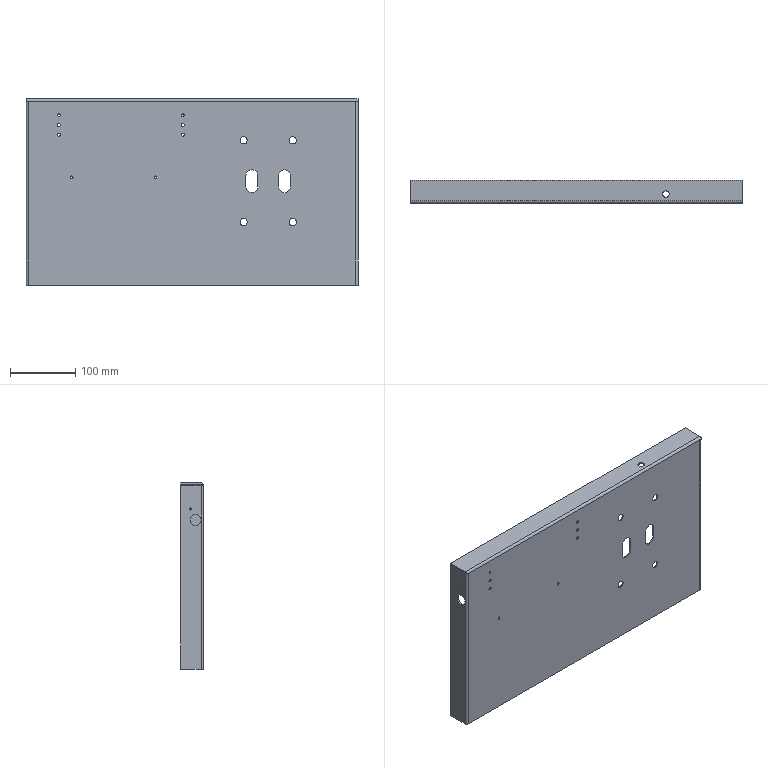Part | STEP file | 5090503 | 1 solid | 51 faces | box 508 x 35 x 285 mm | volume 354091 mm3 | plane 26 | cylinder 25 | commonest cylinder face diameters 4 x4 4.5 x4 11 x4 18 x4 3 x3 7 x3